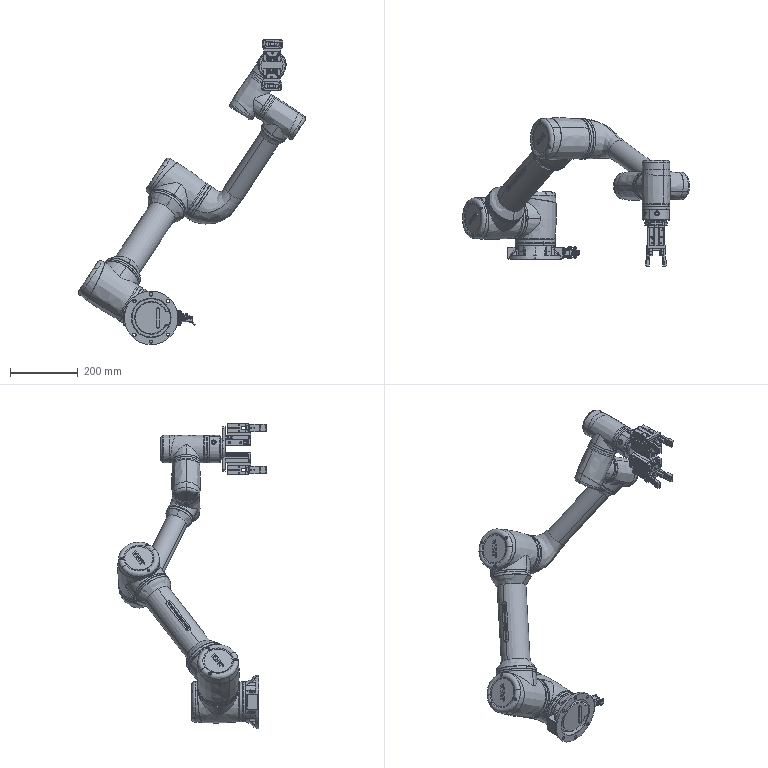Part | SolidWorks | 30 solids | 3504 faces | volume 12699341 mm3 | plane 1762 | cylinder 930 | spline 366 | cone 363 | torus 80 | sphere 3 | commonest cylinder face diameters 4.134 x68 3.242 x64 118 x48 0.4 x44 1 x43 2 x43